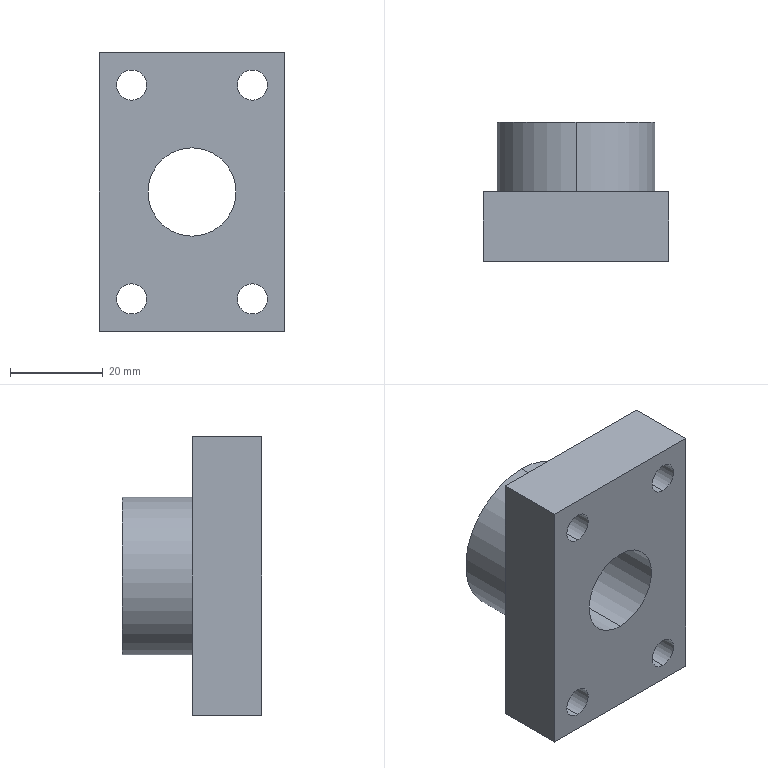Part | STEP file | 1 solid | 19 faces | box 40 x 30 x 60 mm | volume 39122 mm3 | cylinder 12 | plane 7 | commonest cylinder face diameters 6.5 x8 19 x2 34 x2
STEP:
#1=CARTESIAN_POINT('',(0.,0.,0.));
#2=DIRECTION('',(0.,0.,1.));
#3=DIRECTION('',(1.,0.,0.));
#4=AXIS2_PLACEMENT_3D('',#1,#2,#3);
#5=CARTESIAN_POINT('',(-13.,0.,-19.75));
#6=VERTEX_POINT('',#5);
#7=CARTESIAN_POINT('',(-13.,15.,-19.75));
#8=VERTEX_POINT('',#7);
#9=CARTESIAN_POINT('',(-13.,15.,-19.75));
#10=DIRECTION('',(0.,1.,0.));
#11=VECTOR('',#10,1.);
#12=LINE('',#9,#11);
#13=CARTESIAN_POINT('',(-13.,15.,-23.));
#14=DIRECTION('',(0.,1.,0.));
#15=DIRECTION('',(0.,0.,1.));
#16=AXIS2_PLACEMENT_3D('',#13,#14,#15);
#17=CYLINDRICAL_SURFACE('',#16,3.25);
#18=CARTESIAN_POINT('',(6.283,0.));
#19=DIRECTION('',(0.,1.));
#20=VECTOR('',#19,1.);
#21=LINE('',#18,#20);
#22=(GEOMETRIC_REPRESENTATION_CONTEXT(2)PARAMETRIC_REPRESENTATION_CONTEXT()REPRESENTATION_CONTEXT('',''));
#23=DEFINITIONAL_REPRESENTATION('',(#21),#22);
#24=PCURVE('',#17,#23);
#25=CARTESIAN_POINT('',(-13.,15.,-23.));
#26=DIRECTION('',(0.,1.,0.));
#27=DIRECTION('',(0.,0.,1.));
#28=AXIS2_PLACEMENT_3D('',#25,#26,#27);
#29=CYLINDRICAL_SURFACE('',#28,3.25);
#30=CARTESIAN_POINT('',(0.,0.));
#31=DIRECTION('',(0.,1.));
#32=VECTOR('',#31,1.);
#33=LINE('',#30,#32);
#34=(GEOMETRIC_REPRESENTATION_CONTEXT(2)PARAMETRIC_REPRESENTATION_CONTEXT()REPRESENTATION_CONTEXT('',''));
#35=DEFINITIONAL_REPRESENTATION('',(#33),#34);
#36=PCURVE('',#29,#35);
#37=SURFACE_CURVE('',#12,(#24,#36),.PCURVE_S1.);
#38=EDGE_CURVE('',#6,#8,#37,.T.);
#39=ORIENTED_EDGE('',*,*,#38,.T.);
#40=CARTESIAN_POINT('',(-13.,15.,-26.25));
#41=VERTEX_POINT('',#40);
#42=CARTESIAN_POINT('',(-13.,15.,-23.));
#43=DIRECTION('',(0.,1.,0.));
#44=DIRECTION('',(0.,0.,1.));
#45=AXIS2_PLACEMENT_3D('',#42,#43,#44);
#46=CIRCLE('',#45,3.25);
#47=CARTESIAN_POINT('',(0.,0.));
#48=DIRECTION('',(1.,0.));
#49=VECTOR('',#48,1.);
#50=LINE('',#47,#49);
#51=(GEOMETRIC_REPRESENTATION_CONTEXT(2)PARAMETRIC_REPRESENTATION_CONTEXT()REPRESENTATION_CONTEXT('',''));
#52=DEFINITIONAL_REPRESENTATION('',(#50),#51);
#53=PCURVE('',#17,#52);
#54=CARTESIAN_POINT('',(0.,15.,0.));
#55=DIRECTION('',(0.,1.,0.));
#56=DIRECTION('',(0.,0.,1.));
#57=AXIS2_PLACEMENT_3D('',#54,#55,#56);
#58=PLANE('',#57);
#59=CARTESIAN_POINT('',(-23.,-13.));
#60=DIRECTION('',(1.,0.));
#61=AXIS2_PLACEMENT_2D('',#59,#60);
#62=CIRCLE('',#61,3.25);
#63=(GEOMETRIC_REPRESENTATION_CONTEXT(2)PARAMETRIC_REPRESENTATION_CONTEXT()REPRESENTATION_CONTEXT('',''));
#64=DEFINITIONAL_REPRESENTATION('',(#62),#63);
#65=PCURVE('',#58,#64);
#66=SURFACE_CURVE('',#46,(#53,#65),.PCURVE_S1.);
#67=EDGE_CURVE('',#41,#8,#66,.T.);
#68=ORIENTED_EDGE('',*,*,#67,.F.);
#69=CARTESIAN_POINT('',(-13.,0.,-26.25));
#70=VERTEX_POINT('',#69);
#71=CARTESIAN_POINT('',(-13.,15.,-26.25));
#72=DIRECTION('',(0.,1.,0.));
#73=VECTOR('',#72,1.);
#74=LINE('',#71,#73);
#75=CARTESIAN_POINT('',(3.142,0.));
#76=DIRECTION('',(0.,1.));
#77=VECTOR('',#76,1.);
#78=LINE('',#75,#77);
#79=(GEOMETRIC_REPRESENTATION_CONTEXT(2)PARAMETRIC_REPRESENTATION_CONTEXT()REPRESENTATION_CONTEXT('',''));
#80=DEFINITIONAL_REPRESENTATION('',(#78),#79);
#81=PCURVE('',#17,#80);
#82=CARTESIAN_POINT('',(3.142,0.));
#83=DIRECTION('',(0.,1.));
#84=VECTOR('',#83,1.);
#85=LINE('',#82,#84);
#86=(GEOMETRIC_REPRESENTATION_CONTEXT(2)PARAMETRIC_REPRESENTATION_CONTEXT()REPRESENTATION_CONTEXT('',''));
#87=DEFINITIONAL_REPRESENTATION('',(#85),#86);
#88=PCURVE('',#29,#87);
#89=SURFACE_CURVE('',#74,(#81,#88),.PCURVE_S1.);
#90=EDGE_CURVE('',#70,#41,#89,.T.);
#91=ORIENTED_EDGE('',*,*,#90,.F.);
#92=CARTESIAN_POINT('',(-13.,0.,-23.));
#93=DIRECTION('',(0.,1.,0.));
#94=DIRECTION('',(0.,0.,1.));
#95=AXIS2_PLACEMENT_3D('',#92,#93,#94);
#96=CIRCLE('',#95,3.25);
#97=CARTESIAN_POINT('',(0.,-15.));
#98=DIRECTION('',(1.,0.));
#99=VECTOR('',#98,1.);
#100=LINE('',#97,#99);
#101=(GEOMETRIC_REPRESENTATION_CONTEXT(2)PARAMETRIC_REPRESENTATION_CONTEXT()REPRESENTATION_CONTEXT('',''));
#102=DEFINITIONAL_REPRESENTATION('',(#100),#101);
#103=PCURVE('',#17,#102);
#104=CARTESIAN_POINT('',(0.,0.,0.));
#105=DIRECTION('',(0.,1.,0.));
#106=DIRECTION('',(0.,0.,1.));
#107=AXIS2_PLACEMENT_3D('',#104,#105,#106);
#108=PLANE('',#107);
#109=CARTESIAN_POINT('',(-23.,-13.));
#110=DIRECTION('',(1.,0.));
#111=AXIS2_PLACEMENT_2D('',#109,#110);
#112=CIRCLE('',#111,3.25);
#113=(GEOMETRIC_REPRESENTATION_CONTEXT(2)PARAMETRIC_REPRESENTATION_CONTEXT()REPRESENTATION_CONTEXT('',''));
#114=DEFINITIONAL_REPRESENTATION('',(#112),#113);
#115=PCURVE('',#108,#114);
#116=SURFACE_CURVE('',#96,(#103,#115),.PCURVE_S1.);
#117=EDGE_CURVE('',#70,#6,#116,.T.);
#118=ORIENTED_EDGE('',*,*,#117,.T.);
#119=EDGE_LOOP('',(#39,#68,#91,#118));
#120=FACE_BOUND('',#119,.F.);
#121=ADVANCED_FACE('',(#120),#17,.F.);
#122=CARTESIAN_POINT('',(13.,0.,-19.75));
#123=VERTEX_POINT('',#122);
#124=CARTESIAN_POINT('',(13.,15.,-19.75));
#125=VERTEX_POINT('',#124);
#126=CARTESIAN_POINT('',(13.,15.,-19.75));
#127=DIRECTION('',(0.,1.,0.));
#128=VECTOR('',#127,1.);
#129=LINE('',#126,#128);
#130=CARTESIAN_POINT('',(13.,15.,-23.));
#131=DIRECTION('',(0.,1.,0.));
#132=DIRECTION('',(0.,0.,1.));
#133=AXIS2_PLACEMENT_3D('',#130,#131,#132);
#134=CYLINDRICAL_SURFACE('',#133,3.25);
#135=CARTESIAN_POINT('',(6.283,0.));
#136=DIRECTION('',(0.,1.));
#137=VECTOR('',#136,1.);
#138=LINE('',#135,#137);
#139=(GEOMETRIC_REPRESENTATION_CONTEXT(2)PARAMETRIC_REPRESENTATION_CONTEXT()REPRESENTATION_CONTEXT('',''));
#140=DEFINITIONAL_REPRESENTATION('',(#138),#139);
#141=PCURVE('',#134,#140);
#142=CARTESIAN_POINT('',(13.,15.,-23.));
#143=DIRECTION('',(0.,1.,0.));
#144=DIRECTION('',(0.,0.,1.));
#145=AXIS2_PLACEMENT_3D('',#142,#143,#144);
#146=CYLINDRICAL_SURFACE('',#145,3.25);
#147=CARTESIAN_POINT('',(0.,0.));
#148=DIRECTION('',(0.,1.));
#149=VECTOR('',#148,1.);
#150=LINE('',#147,#149);
#151=(GEOMETRIC_REPRESENTATION_CONTEXT(2)PARAMETRIC_REPRESENTATION_CONTEXT()REPRESENTATION_CONTEXT('',''));
#152=DEFINITIONAL_REPRESENTATION('',(#150),#151);
#153=PCURVE('',#146,#152);
#154=SURFACE_CURVE('',#129,(#141,#153),.PCURVE_S1.);
#155=EDGE_CURVE('',#123,#125,#154,.T.);
#156=ORIENTED_EDGE('',*,*,#155,.T.);
#157=CARTESIAN_POINT('',(13.,15.,-26.25));
#158=VERTEX_POINT('',#157);
#159=CARTESIAN_POINT('',(13.,15.,-23.));
#160=DIRECTION('',(0.,1.,0.));
#161=DIRECTION('',(0.,0.,1.));
#162=AXIS2_PLACEMENT_3D('',#159,#160,#161);
#163=CIRCLE('',#162,3.25);
#164=CARTESIAN_POINT('',(0.,0.));
#165=DIRECTION('',(1.,0.));
#166=VECTOR('',#165,1.);
#167=LINE('',#164,#166);
#168=(GEOMETRIC_REPRESENTATION_CONTEXT(2)PARAMETRIC_REPRESENTATION_CONTEXT()REPRESENTATION_CONTEXT('',''));
#169=DEFINITIONAL_REPRESENTATION('',(#167),#168);
#170=PCURVE('',#134,#169);
#171=CARTESIAN_POINT('',(-23.,13.));
#172=DIRECTION('',(1.,0.));
#173=AXIS2_PLACEMENT_2D('',#171,#172);
#174=CIRCLE('',#173,3.25);
#175=(GEOMETRIC_REPRESENTATION_CONTEXT(2)PARAMETRIC_REPRESENTATION_CONTEXT()REPRESENTATION_CONTEXT('',''));
#176=DEFINITIONAL_REPRESENTATION('',(#174),#175);
#177=PCURVE('',#58,#176);
#178=SURFACE_CURVE('',#163,(#170,#177),.PCURVE_S1.);
#179=EDGE_CURVE('',#158,#125,#178,.T.);
#180=ORIENTED_EDGE('',*,*,#179,.F.);
#181=CARTESIAN_POINT('',(13.,0.,-26.25));
#182=VERTEX_POINT('',#181);
#183=CARTESIAN_POINT('',(13.,15.,-26.25));
#184=DIRECTION('',(0.,1.,0.));
#185=VECTOR('',#184,1.);
#186=LINE('',#183,#185);
#187=CARTESIAN_POINT('',(3.142,0.));
#188=DIRECTION('',(0.,1.));
#189=VECTOR('',#188,1.);
#190=LINE('',#187,#189);
#191=(GEOMETRIC_REPRESENTATION_CONTEXT(2)PARAMETRIC_REPRESENTATION_CONTEXT()REPRESENTATION_CONTEXT('',''));
#192=DEFINITIONAL_REPRESENTATION('',(#190),#191);
#193=PCURVE('',#134,#192);
#194=CARTESIAN_POINT('',(3.142,0.));
#195=DIRECTION('',(0.,1.));
#196=VECTOR('',#195,1.);
#197=LINE('',#194,#196);
#198=(GEOMETRIC_REPRESENTATION_CONTEXT(2)PARAMETRIC_REPRESENTATION_CONTEXT()REPRESENTATION_CONTEXT('',''));
#199=DEFINITIONAL_REPRESENTATION('',(#197),#198);
#200=PCURVE('',#146,#199);
#201=SURFACE_CURVE('',#186,(#193,#200),.PCURVE_S1.);
#202=EDGE_CURVE('',#182,#158,#201,.T.);
#203=ORIENTED_EDGE('',*,*,#202,.F.);
#204=CARTESIAN_POINT('',(13.,0.,-23.));
#205=DIRECTION('',(0.,1.,0.));
#206=DIRECTION('',(0.,0.,1.));
#207=AXIS2_PLACEMENT_3D('',#204,#205,#206);
#208=CIRCLE('',#207,3.25);
#209=CARTESIAN_POINT('',(0.,-15.));
#210=DIRECTION('',(1.,0.));
#211=VECTOR('',#210,1.);
#212=LINE('',#209,#211);
#213=(GEOMETRIC_REPRESENTATION_CONTEXT(2)PARAMETRIC_REPRESENTATION_CONTEXT()REPRESENTATION_CONTEXT('',''));
#214=DEFINITIONAL_REPRESENTATION('',(#212),#213);
#215=PCURVE('',#134,#214);
#216=CARTESIAN_POINT('',(-23.,13.));
#217=DIRECTION('',(1.,0.));
#218=AXIS2_PLACEMENT_2D('',#216,#217);
#219=CIRCLE('',#218,3.25);
#220=(GEOMETRIC_REPRESENTATION_CONTEXT(2)PARAMETRIC_REPRESENTATION_CONTEXT()REPRESENTATION_CONTEXT('',''));
#221=DEFINITIONAL_REPRESENTATION('',(#219),#220);
#222=PCURVE('',#108,#221);
#223=SURFACE_CURVE('',#208,(#215,#222),.PCURVE_S1.);
#224=EDGE_CURVE('',#182,#123,#223,.T.);
#225=ORIENTED_EDGE('',*,*,#224,.T.);
#226=EDGE_LOOP('',(#156,#180,#203,#225));
#227=FACE_BOUND('',#226,.F.);
#228=ADVANCED_FACE('',(#227),#134,.F.);
#229=CARTESIAN_POINT('',(13.,0.,26.25));
#230=VERTEX_POINT('',#229);
#231=CARTESIAN_POINT('',(13.,15.,26.25));
#232=VERTEX_POINT('',#231);
#233=CARTESIAN_POINT('',(13.,15.,26.25));
#234=DIRECTION('',(0.,1.,0.));
#235=VECTOR('',#234,1.);
#236=LINE('',#233,#235);
#237=CARTESIAN_POINT('',(13.,15.,23.));
#238=DIRECTION('',(0.,1.,0.));
#239=DIRECTION('',(0.,0.,1.));
#240=AXIS2_PLACEMENT_3D('',#237,#238,#239);
#241=CYLINDRICAL_SURFACE('',#240,3.25);
#242=CARTESIAN_POINT('',(6.283,0.));
#243=DIRECTION('',(0.,1.));
#244=VECTOR('',#243,1.);
#245=LINE('',#242,#244);
#246=(GEOMETRIC_REPRESENTATION_CONTEXT(2)PARAMETRIC_REPRESENTATION_CONTEXT()REPRESENTATION_CONTEXT('',''));
#247=DEFINITIONAL_REPRESENTATION('',(#245),#246);
#248=PCURVE('',#241,#247);
#249=CARTESIAN_POINT('',(13.,15.,23.));
#250=DIRECTION('',(0.,1.,0.));
#251=DIRECTION('',(0.,0.,1.));
#252=AXIS2_PLACEMENT_3D('',#249,#250,#251);
#253=CYLINDRICAL_SURFACE('',#252,3.25);
#254=CARTESIAN_POINT('',(0.,0.));
#255=DIRECTION('',(0.,1.));
#256=VECTOR('',#255,1.);
#257=LINE('',#254,#256);
#258=(GEOMETRIC_REPRESENTATION_CONTEXT(2)PARAMETRIC_REPRESENTATION_CONTEXT()REPRESENTATION_CONTEXT('',''));
#259=DEFINITIONAL_REPRESENTATION('',(#257),#258);
#260=PCURVE('',#253,#259);
#261=SURFACE_CURVE('',#236,(#248,#260),.PCURVE_S1.);
#262=EDGE_CURVE('',#230,#232,#261,.T.);
#263=ORIENTED_EDGE('',*,*,#262,.T.);
#264=CARTESIAN_POINT('',(13.,15.,19.75));
#265=VERTEX_POINT('',#264);
#266=CARTESIAN_POINT('',(13.,15.,23.));
#267=DIRECTION('',(0.,1.,0.));
#268=DIRECTION('',(0.,0.,1.));
#269=AXIS2_PLACEMENT_3D('',#266,#267,#268);
#270=CIRCLE('',#269,3.25);
#271=CARTESIAN_POINT('',(0.,0.));
#272=DIRECTION('',(1.,0.));
#273=VECTOR('',#272,1.);
#274=LINE('',#271,#273);
#275=(GEOMETRIC_REPRESENTATION_CONTEXT(2)PARAMETRIC_REPRESENTATION_CONTEXT()REPRESENTATION_CONTEXT('',''));
#276=DEFINITIONAL_REPRESENTATION('',(#274),#275);
#277=PCURVE('',#241,#276);
#278=CARTESIAN_POINT('',(23.,13.));
#279=DIRECTION('',(1.,0.));
#280=AXIS2_PLACEMENT_2D('',#278,#279);
#281=CIRCLE('',#280,3.25);
#282=(GEOMETRIC_REPRESENTATION_CONTEXT(2)PARAMETRIC_REPRESENTATION_CONTEXT()REPRESENTATION_CONTEXT('',''));
#283=DEFINITIONAL_REPRESENTATION('',(#281),#282);
#284=PCURVE('',#58,#283);
#285=SURFACE_CURVE('',#270,(#277,#284),.PCURVE_S1.);
#286=EDGE_CURVE('',#265,#232,#285,.T.);
#287=ORIENTED_EDGE('',*,*,#286,.F.);
#288=CARTESIAN_POINT('',(13.,0.,19.75));
#289=VERTEX_POINT('',#288);
#290=CARTESIAN_POINT('',(13.,15.,19.75));
#291=DIRECTION('',(0.,1.,0.));
#292=VECTOR('',#291,1.);
#293=LINE('',#290,#292);
#294=CARTESIAN_POINT('',(3.142,0.));
#295=DIRECTION('',(0.,1.));
#296=VECTOR('',#295,1.);
#297=LINE('',#294,#296);
#298=(GEOMETRIC_REPRESENTATION_CONTEXT(2)PARAMETRIC_REPRESENTATION_CONTEXT()REPRESENTATION_CONTEXT('',''));
#299=DEFINITIONAL_REPRESENTATION('',(#297),#298);
#300=PCURVE('',#241,#299);
#301=CARTESIAN_POINT('',(3.142,0.));
#302=DIRECTION('',(0.,1.));
#303=VECTOR('',#302,1.);
#304=LINE('',#301,#303);
#305=(GEOMETRIC_REPRESENTATION_CONTEXT(2)PARAMETRIC_REPRESENTATION_CONTEXT()REPRESENTATION_CONTEXT('',''));
#306=DEFINITIONAL_REPRESENTATION('',(#304),#305);
#307=PCURVE('',#253,#306);
#308=SURFACE_CURVE('',#293,(#300,#307),.PCURVE_S1.);
#309=EDGE_CURVE('',#289,#265,#308,.T.);
#310=ORIENTED_EDGE('',*,*,#309,.F.);
#311=CARTESIAN_POINT('',(13.,0.,23.));
#312=DIRECTION('',(0.,1.,0.));
#313=DIRECTION('',(0.,0.,1.));
#314=AXIS2_PLACEMENT_3D('',#311,#312,#313);
#315=CIRCLE('',#314,3.25);
#316=CARTESIAN_POINT('',(0.,-15.));
#317=DIRECTION('',(1.,0.));
#318=VECTOR('',#317,1.);
#319=LINE('',#316,#318);
#320=(GEOMETRIC_REPRESENTATION_CONTEXT(2)PARAMETRIC_REPRESENTATION_CONTEXT()REPRESENTATION_CONTEXT('',''));
#321=DEFINITIONAL_REPRESENTATION('',(#319),#320);
#322=PCURVE('',#241,#321);
#323=CARTESIAN_POINT('',(23.,13.));
#324=DIRECTION('',(1.,0.));
#325=AXIS2_PLACEMENT_2D('',#323,#324);
#326=CIRCLE('',#325,3.25);
#327=(GEOMETRIC_REPRESENTATION_CONTEXT(2)PARAMETRIC_REPRESENTATION_CONTEXT()REPRESENTATION_CONTEXT('',''));
#328=DEFINITIONAL_REPRESENTATION('',(#326),#327);
#329=PCURVE('',#108,#328);
#330=SURFACE_CURVE('',#315,(#322,#329),.PCURVE_S1.);
#331=EDGE_CURVE('',#289,#230,#330,.T.);
#332=ORIENTED_EDGE('',*,*,#331,.T.);
#333=EDGE_LOOP('',(#263,#287,#310,#332));
#334=FACE_BOUND('',#333,.F.);
#335=ADVANCED_FACE('',(#334),#241,.F.);
#336=CARTESIAN_POINT('',(-13.,0.,26.25));
#337=VERTEX_POINT('',#336);
#338=CARTESIAN_POINT('',(-13.,15.,26.25));
#339=VERTEX_POINT('',#338);
#340=CARTESIAN_POINT('',(-13.,15.,26.25));
#341=DIRECTION('',(0.,1.,0.));
#342=VECTOR('',#341,1.);
#343=LINE('',#340,#342);
#344=CARTESIAN_POINT('',(-13.,15.,23.));
#345=DIRECTION('',(0.,1.,0.));
#346=DIRECTION('',(0.,0.,1.));
#347=AXIS2_PLACEMENT_3D('',#344,#345,#346);
#348=CYLINDRICAL_SURFACE('',#347,3.25);
#349=CARTESIAN_POINT('',(6.283,0.));
#350=DIRECTION('',(0.,1.));
#351=VECTOR('',#350,1.);
#352=LINE('',#349,#351);
#353=(GEOMETRIC_REPRESENTATION_CONTEXT(2)PARAMETRIC_REPRESENTATION_CONTEXT()REPRESENTATION_CONTEXT('',''));
#354=DEFINITIONAL_REPRESENTATION('',(#352),#353);
#355=PCURVE('',#348,#354);
#356=CARTESIAN_POINT('',(-13.,15.,23.));
#357=DIRECTION('',(0.,1.,0.));
#358=DIRECTION('',(0.,0.,1.));
#359=AXIS2_PLACEMENT_3D('',#356,#357,#358);
#360=CYLINDRICAL_SURFACE('',#359,3.25);
#361=CARTESIAN_POINT('',(0.,0.));
#362=DIRECTION('',(0.,1.));
#363=VECTOR('',#362,1.);
#364=LINE('',#361,#363);
#365=(GEOMETRIC_REPRESENTATION_CONTEXT(2)PARAMETRIC_REPRESENTATION_CONTEXT()REPRESENTATION_CONTEXT('',''));
#366=DEFINITIONAL_REPRESENTATION('',(#364),#365);
#367=PCURVE('',#360,#366);
#368=SURFACE_CURVE('',#343,(#355,#367),.PCURVE_S1.);
#369=EDGE_CURVE('',#337,#339,#368,.T.);
#370=ORIENTED_EDGE('',*,*,#369,.T.);
#371=CARTESIAN_POINT('',(-13.,15.,19.75));
#372=VERTEX_POINT('',#371);
#373=CARTESIAN_POINT('',(-13.,15.,23.));
#374=DIRECTION('',(0.,1.,0.));
#375=DIRECTION('',(0.,0.,1.));
#376=AXIS2_PLACEMENT_3D('',#373,#374,#375);
#377=CIRCLE('',#376,3.25);
#378=CARTESIAN_POINT('',(0.,0.));
#379=DIRECTION('',(1.,0.));
#380=VECTOR('',#379,1.);
#381=LINE('',#378,#380);
#382=(GEOMETRIC_REPRESENTATION_CONTEXT(2)PARAMETRIC_REPRESENTATION_CONTEXT()REPRESENTATION_CONTEXT('',''));
#383=DEFINITIONAL_REPRESENTATION('',(#381),#382);
#384=PCURVE('',#348,#383);
#385=CARTESIAN_POINT('',(23.,-13.));
#386=DIRECTION('',(1.,0.));
#387=AXIS2_PLACEMENT_2D('',#385,#386);
#388=CIRCLE('',#387,3.25);
#389=(GEOMETRIC_REPRESENTATION_CONTEXT(2)PARAMETRIC_REPRESENTATION_CONTEXT()REPRESENTATION_CONTEXT('',''));
#390=DEFINITIONAL_REPRESENTATION('',(#388),#389);
#391=PCURVE('',#58,#390);
#392=SURFACE_CURVE('',#377,(#384,#391),.PCURVE_S1.);
#393=EDGE_CURVE('',#372,#339,#392,.T.);
#394=ORIENTED_EDGE('',*,*,#393,.F.);
#395=CARTESIAN_POINT('',(-13.,0.,19.75));
#396=VERTEX_POINT('',#395);
#397=CARTESIAN_POINT('',(-13.,15.,19.75));
#398=DIRECTION('',(0.,1.,0.));
#399=VECTOR('',#398,1.);
#400=LINE('',#397,#399);
#401=CARTESIAN_POINT('',(3.142,0.));
#402=DIRECTION('',(0.,1.));
#403=VECTOR('',#402,1.);
#404=LINE('',#401,#403);
#405=(GEOMETRIC_REPRESENTATION_CONTEXT(2)PARAMETRIC_REPRESENTATION_CONTEXT()REPRESENTATION_CONTEXT('',''));
#406=DEFINITIONAL_REPRESENTATION('',(#404),#405);
#407=PCURVE('',#348,#406);
#408=CARTESIAN_POINT('',(3.142,0.));
#409=DIRECTION('',(0.,1.));
#410=VECTOR('',#409,1.);
#411=LINE('',#408,#410);
#412=(GEOMETRIC_REPRESENTATION_CONTEXT(2)PARAMETRIC_REPRESENTATION_CONTEXT()REPRESENTATION_CONTEXT('',''));
#413=DEFINITIONAL_REPRESENTATION('',(#411),#412);
#414=PCURVE('',#360,#413);
#415=SURFACE_CURVE('',#400,(#407,#414),.PCURVE_S1.);
#416=EDGE_CURVE('',#396,#372,#415,.T.);
#417=ORIENTED_EDGE('',*,*,#416,.F.);
#418=CARTESIAN_POINT('',(-13.,0.,23.));
#419=DIRECTION('',(0.,1.,0.));
#420=DIRECTION('',(0.,0.,1.));
#421=AXIS2_PLACEMENT_3D('',#418,#419,#420);
#422=CIRCLE('',#421,3.25);
#423=CARTESIAN_POINT('',(0.,-15.));
#424=DIRECTION('',(1.,0.));
#425=VECTOR('',#424,1.);
#426=LINE('',#423,#425);
#427=(GEOMETRIC_REPRESENTATION_CONTEXT(2)PARAMETRIC_REPRESENTATION_CONTEXT()REPRESENTATION_CONTEXT('',''));
#428=DEFINITIONAL_REPRESENTATION('',(#426),#427);
#429=PCURVE('',#348,#428);
#430=CARTESIAN_POINT('',(23.,-13.));
#431=DIRECTION('',(1.,0.));
#432=AXIS2_PLACEMENT_2D('',#430,#431);
#433=CIRCLE('',#432,3.25);
#434=(GEOMETRIC_REPRESENTATION_CONTEXT(2)PARAMETRIC_REPRESENTATION_CONTEXT()REPRESENTATION_CONTEXT('',''));
#435=DEFINITIONAL_REPRESENTATION('',(#433),#434);
#436=PCURVE('',#108,#435);
#437=SURFACE_CURVE('',#422,(#429,#436),.PCURVE_S1.);
#438=EDGE_CURVE('',#396,#337,#437,.T.);
#439=ORIENTED_EDGE('',*,*,#438,.T.);
#440=EDGE_LOOP('',(#370,#394,#417,#439));
#441=FACE_BOUND('',#440,.F.);
#442=ADVANCED_FACE('',(#441),#348,.F.);
#443=CARTESIAN_POINT('',(0.,0.,9.5));
#444=VERTEX_POINT('',#443);
#445=CARTESIAN_POINT('',(0.,30.,9.5));
#446=VERTEX_POINT('',#445);
#447=CARTESIAN_POINT('',(0.,0.,9.5));
#448=DIRECTION('',(0.,1.,0.));
#449=VECTOR('',#448,1.);
#450=LINE('',#447,#449);
#451=CARTESIAN_POINT('',(0.,0.,0.));
#452=DIRECTION('',(0.,1.,0.));
#453=DIRECTION('',(0.,0.,1.));
#454=AXIS2_PLACEMENT_3D('',#451,#452,#453);
#455=CYLINDRICAL_SURFACE('',#454,9.5);
#456=CARTESIAN_POINT('',(6.283,0.));
#457=DIRECTION('',(0.,1.));
#458=VECTOR('',#457,1.);
#459=LINE('',#456,#458);
#460=(GEOMETRIC_REPRESENTATION_CONTEXT(2)PARAMETRIC_REPRESENTATION_CONTEXT()REPRESENTATION_CONTEXT('',''));
#461=DEFINITIONAL_REPRESENTATION('',(#459),#460);
#462=PCURVE('',#455,#461);
#463=CARTESIAN_POINT('',(0.,0.,0.));
#464=DIRECTION('',(0.,1.,0.));
#465=DIRECTION('',(0.,0.,1.));
#466=AXIS2_PLACEMENT_3D('',#463,#464,#465);
#467=CYLINDRICAL_SURFACE('',#466,9.5);
#468=CARTESIAN_POINT('',(0.,0.));
#469=DIRECTION('',(0.,1.));
#470=VECTOR('',#469,1.);
#471=LINE('',#468,#470);
#472=(GEOMETRIC_REPRESENTATION_CONTEXT(2)PARAMETRIC_REPRESENTATION_CONTEXT()REPRESENTATION_CONTEXT('',''));
#473=DEFINITIONAL_REPRESENTATION('',(#471),#472);
#474=PCURVE('',#467,#473);
#475=SURFACE_CURVE('',#450,(#462,#474),.PCURVE_S1.);
#476=EDGE_CURVE('',#444,#446,#475,.T.);
#477=ORIENTED_EDGE('',*,*,#476,.T.);
#478=CARTESIAN_POINT('',(0.,30.,-9.5));
#479=VERTEX_POINT('',#478);
#480=CARTESIAN_POINT('',(0.,30.,0.));
#481=DIRECTION('',(0.,1.,0.));
#482=DIRECTION('',(0.,0.,1.));
#483=AXIS2_PLACEMENT_3D('',#480,#481,#482);
#484=CIRCLE('',#483,9.5);
#485=CARTESIAN_POINT('',(0.,30.));
#486=DIRECTION('',(1.,0.));
#487=VECTOR('',#486,1.);
#488=LINE('',#485,#487);
#489=(GEOMETRIC_REPRESENTATION_CONTEXT(2)PARAMETRIC_REPRESENTATION_CONTEXT()REPRESENTATION_CONTEXT('',''));
#490=DEFINITIONAL_REPRESENTATION('',(#488),#489);
#491=PCURVE('',#455,#490);
#492=CARTESIAN_POINT('',(0.,30.,0.));
#493=DIRECTION('',(0.,1.,0.));
#494=DIRECTION('',(0.,0.,1.));
#495=AXIS2_PLACEMENT_3D('',#492,#493,#494);
#496=PLANE('',#495);
#497=CARTESIAN_POINT('',(0.,0.));
#498=DIRECTION('',(1.,0.));
#499=AXIS2_PLACEMENT_2D('',#497,#498);
#500=CIRCLE('',#499,9.5);
#501=(GEOMETRIC_REPRESENTATION_CONTEXT(2)PARAMETRIC_REPRESENTATION_CONTEXT()REPRESENTATION_CONTEXT('',''));
#502=DEFINITIONAL_REPRESENTATION('',(#500),#501);
#503=PCURVE('',#496,#502);
#504=SURFACE_CURVE('',#484,(#491,#503),.PCURVE_S1.);
#505=EDGE_CURVE('',#479,#446,#504,.T.);
#506=ORIENTED_EDGE('',*,*,#505,.F.);
#507=CARTESIAN_POINT('',(0.,0.,-9.5));
#508=VERTEX_POINT('',#507);
#509=CARTESIAN_POINT('',(0.,0.,-9.5));
#510=DIRECTION('',(0.,1.,0.));
#511=VECTOR('',#510,1.);
#512=LINE('',#509,#511);
#513=CARTESIAN_POINT('',(3.142,0.));
#514=DIRECTION('',(0.,1.));
#515=VECTOR('',#514,1.);
#516=LINE('',#513,#515);
#517=(GEOMETRIC_REPRESENTATION_CONTEXT(2)PARAMETRIC_REPRESENTATION_CONTEXT()REPRESENTATION_CONTEXT('',''));
#518=DEFINITIONAL_REPRESENTATION('',(#516),#517);
#519=PCURVE('',#455,#518);
#520=CARTESIAN_POINT('',(3.142,0.));
#521=DIRECTION('',(0.,1.));
#522=VECTOR('',#521,1.);
#523=LINE('',#520,#522);
#524=(GEOMETRIC_REPRESENTATION_CONTEXT(2)PARAMETRIC_REPRESENTATION_CONTEXT()REPRESENTATION_CONTEXT('',''));
#525=DEFINITIONAL_REPRESENTATION('',(#523),#524);
#526=PCURVE('',#467,#525);
#527=SURFACE_CURVE('',#512,(#519,#526),.PCURVE_S1.);
#528=EDGE_CURVE('',#508,#479,#527,.T.);
#529=ORIENTED_EDGE('',*,*,#528,.F.);
#530=CARTESIAN_POINT('',(0.,0.,0.));
#531=DIRECTION('',(0.,1.,0.));
#532=DIRECTION('',(0.,0.,1.));
#533=AXIS2_PLACEMENT_3D('',#530,#531,#532);
#534=CIRCLE('',#533,9.5);
#535=CARTESIAN_POINT('',(0.,0.));
#536=DIRECTION('',(1.,0.));
#537=VECTOR('',#536,1.);
#538=LINE('',#535,#537);
#539=(GEOMETRIC_REPRESENTATION_CONTEXT(2)PARAMETRIC_REPRESENTATION_CONTEXT()REPRESENTATION_CONTEXT('',''));
#540=DEFINITIONAL_REPRESENTATION('',(#538),#539);
#541=PCURVE('',#455,#540);
#542=CARTESIAN_POINT('',(0.,0.));
#543=DIRECTION('',(1.,0.));
#544=AXIS2_PLACEMENT_2D('',#542,#543);
#545=CIRCLE('',#544,9.5);
#546=(GEOMETRIC_REPRESENTATION_CONTEXT(2)PARAMETRIC_REPRESENTATION_CONTEXT()REPRESENTATION_CONTEXT('',''));
#547=DEFINITIONAL_REPRESENTATION('',(#545),#546);
#548=PCURVE('',#108,#547);
#549=SURFACE_CURVE('',#534,(#541,#548),.PCURVE_S1.);
#550=EDGE_CURVE('',#508,#444,#549,.T.);
#551=ORIENTED_EDGE('',*,*,#550,.T.);
#552=EDGE_LOOP('',(#477,#506,#529,#551));
#553=FACE_BOUND('',#552,.F.);
#554=ADVANCED_FACE('',(#553),#455,.F.);
#555=CARTESIAN_POINT('',(0.,30.,17.));
#556=VERTEX_POINT('',#555);
#557=CARTESIAN_POINT('',(0.,30.,-17.));
#558=VERTEX_POINT('',#557);
#559=CARTESIAN_POINT('',(0.,30.,0.));
#560=DIRECTION('',(0.,1.,0.));
#561=DIRECTION('',(0.,0.,1.));
#562=AXIS2_PLACEMENT_3D('',#559,#560,#561);
#563=CIRCLE('',#562,17.);
#564=CARTESIAN_POINT('',(0.,30.,0.));
#565=DIRECTION('',(0.,-1.,0.));
#566=DIRECTION('',(0.,0.,-1.));
#567=AXIS2_PLACEMENT_3D('',#564,#565,#566);
#568=CYLINDRICAL_SURFACE('',#567,17.);
#569=CARTESIAN_POINT('',(3.142,0.));
#570=DIRECTION('',(-1.,0.));
#571=VECTOR('',#570,1.);
#572=LINE('',#569,#571);
#573=(GEOMETRIC_REPRESENTATION_CONTEXT(2)PARAMETRIC_REPRESENTATION_CONTEXT()REPRESENTATION_CONTEXT('',''));
#574=DEFINITIONAL_REPRESENTATION('',(#572),#573);
#575=PCURVE('',#568,#574);
#576=CARTESIAN_POINT('',(0.,0.));
#577=DIRECTION('',(1.,0.));
#578=AXIS2_PLACEMENT_2D('',#576,#577);
#579=CIRCLE('',#578,17.);
#580=(GEOMETRIC_REPRESENTATION_CONTEXT(2)PARAMETRIC_REPRESENTATION_CONTEXT()REPRESENTATION_CONTEXT('',''));
#581=DEFINITIONAL_REPRESENTATION('',(#579),#580);
#582=PCURVE('',#496,#581);
#583=SURFACE_CURVE('',#563,(#575,#582),.PCURVE_S1.);
#584=EDGE_CURVE('',#556,#558,#583,.T.);
#585=ORIENTED_EDGE('',*,*,#584,.F.);
#586=CARTESIAN_POINT('',(0.,15.,17.));
#587=VERTEX_POINT('',#586);
#588=CARTESIAN_POINT('',(0.,30.,17.));
#589=DIRECTION('',(0.,-1.,0.));
#590=VECTOR('',#589,1.);
#591=LINE('',#588,#590);
#592=CARTESIAN_POINT('',(3.142,0.));
#593=DIRECTION('',(0.,1.));
#594=VECTOR('',#593,1.);
#595=LINE('',#592,#594);
#596=(GEOMETRIC_REPRESENTATION_CONTEXT(2)PARAMETRIC_REPRESENTATION_CONTEXT()REPRESENTATION_CONTEXT('',''));
#597=DEFINITIONAL_REPRESENTATION('',(#595),#596);
#598=PCURVE('',#568,#597);
#599=CARTESIAN_POINT('',(0.,30.,0.));
#600=DIRECTION('',(0.,-1.,0.));
#601=DIRECTION('',(0.,0.,-1.));
#602=AXIS2_PLACEMENT_3D('',#599,#600,#601);
#603=CYLINDRICAL_SURFACE('',#602,17.);
#604=CARTESIAN_POINT('',(3.142,0.));
#605=DIRECTION('',(0.,1.));
#606=VECTOR('',#605,1.);
#607=LINE('',#604,#606);
#608=(GEOMETRIC_REPRESENTATION_CONTEXT(2)PARAMETRIC_REPRESENTATION_CONTEXT()REPRESENTATION_CONTEXT('',''));
#609=DEFINITIONAL_REPRESENTATION('',(#607),#608);
#610=PCURVE('',#603,#609);
#611=SURFACE_CURVE('',#591,(#598,#610),.PCURVE_S1.);
#612=EDGE_CURVE('',#556,#587,#611,.T.);
#613=ORIENTED_EDGE('',*,*,#612,.T.);
#614=CARTESIAN_POINT('',(0.,15.,-17.));
#615=VERTEX_POINT('',#614);
#616=CARTESIAN_POINT('',(0.,15.,0.));
#617=DIRECTION('',(0.,1.,0.));
#618=DIRECTION('',(0.,0.,1.));
#619=AXIS2_PLACEMENT_3D('',#616,#617,#618);
#620=CIRCLE('',#619,17.);
#621=CARTESIAN_POINT('',(3.142,15.));
#622=DIRECTION('',(-1.,0.));
#623=VECTOR('',#622,1.);
#624=LINE('',#621,#623);
#625=(GEOMETRIC_REPRESENTATION_CONTEXT(2)PARAMETRIC_REPRESENTATION_CONTEXT()REPRESENTATION_CONTEXT('',''));
#626=DEFINITIONAL_REPRESENTATION('',(#624),#625);
#627=PCURVE('',#568,#626);
#628=CARTESIAN_POINT('',(0.,0.));
#629=DIRECTION('',(1.,0.));
#630=AXIS2_PLACEMENT_2D('',#628,#629);
#631=CIRCLE('',#630,17.);
#632=(GEOMETRIC_REPRESENTATION_CONTEXT(2)PARAMETRIC_REPRESENTATION_CONTEXT()REPRESENTATION_CONTEXT('',''));
#633=DEFINITIONAL_REPRESENTATION('',(#631),#632);
#634=PCURVE('',#58,#633);
#635=SURFACE_CURVE('',#620,(#627,#634),.PCURVE_S1.);
#636=EDGE_CURVE('',#587,#615,#635,.T.);
#637=ORIENTED_EDGE('',*,*,#636,.T.);
#638=CARTESIAN_POINT('',(0.,30.,-17.));
#639=DIRECTION('',(0.,-1.,0.));
#640=VECTOR('',#639,1.);
#641=LINE('',#638,#640);
#642=CARTESIAN_POINT('',(0.,0.));
#643=DIRECTION('',(0.,1.));
#644=VECTOR('',#643,1.);
#645=LINE('',#642,#644);
#646=(GEOMETRIC_REPRESENTATION_CONTEXT(2)PARAMETRIC_REPRESENTATION_CONTEXT()REPRESENTATION_CONTEXT('',''));
#647=DEFINITIONAL_REPRESENTATION('',(#645),#646);
#648=PCURVE('',#568,#647);
#649=CARTESIAN_POINT('',(6.283,0.));
#650=DIRECTION('',(0.,1.));
#651=VECTOR('',#650,1.);
#652=LINE('',#649,#651);
#653=(GEOMETRIC_REPRESENTATION_CONTEXT(2)PARAMETRIC_REPRESENTATION_CONTEXT()REPRESENTATION_CONTEXT('',''));
#654=DEFINITIONAL_REPRESENTATION('',(#652),#653);
#655=PCURVE('',#603,#654);
#656=SURFACE_CURVE('',#641,(#648,#655),.PCURVE_S1.);
#657=EDGE_CURVE('',#558,#615,#656,.T.);
#658=ORIENTED_EDGE('',*,*,#657,.F.);
#659=EDGE_LOOP('',(#585,#613,#637,#658));
#660=FACE_BOUND('',#659,.T.);
#661=ADVANCED_FACE('',(#660),#568,.T.);
#662=CARTESIAN_POINT('',(-13.,15.,-23.));
#663=DIRECTION('',(0.,1.,0.));
#664=DIRECTION('',(0.,0.,1.));
#665=AXIS2_PLACEMENT_3D('',#662,#663,#664);
#666=CIRCLE('',#665,3.25);
#667=CARTESIAN_POINT('',(-23.,-13.));
#668=DIRECTION('',(1.,0.));
#669=AXIS2_PLACEMENT_2D('',#667,#668);
#670=CIRCLE('',#669,3.25);
#671=(GEOMETRIC_REPRESENTATION_CONTEXT(2)PARAMETRIC_REPRESENTATION_CONTEXT()REPRESENTATION_CONTEXT('',''));
#672=DEFINITIONAL_REPRESENTATION('',(#670),#671);
#673=PCURVE('',#58,#672);
#674=CARTESIAN_POINT('',(0.,0.));
#675=DIRECTION('',(1.,0.));
#676=VECTOR('',#675,1.);
#677=LINE('',#674,#676);
#678=(GEOMETRIC_REPRESENTATION_CONTEXT(2)PARAMETRIC_REPRESENTATION_CONTEXT()REPRESENTATION_CONTEXT('',''));
#679=DEFINITIONAL_REPRESENTATION('',(#677),#678);
#680=PCURVE('',#29,#679);
#681=SURFACE_CURVE('',#666,(#673,#680),.PCURVE_S1.);
#682=EDGE_CURVE('',#8,#41,#681,.T.);
#683=ORIENTED_EDGE('',*,*,#682,.F.);
#684=ORIENTED_EDGE('',*,*,#67,.F.);
#685=EDGE_LOOP('',(#683,#684));
#686=FACE_BOUND('',#685,.T.);
#687=CARTESIAN_POINT('',(13.,15.,-23.));
#688=DIRECTION('',(0.,1.,0.));
#689=DIRECTION('',(0.,0.,1.));
#690=AXIS2_PLACEMENT_3D('',#687,#688,#689);
#691=CIRCLE('',#690,3.25);
#692=CARTESIAN_POINT('',(-23.,13.));
#693=DIRECTION('',(1.,0.));
#694=AXIS2_PLACEMENT_2D('',#692,#693);
#695=CIRCLE('',#694,3.25);
#696=(GEOMETRIC_REPRESENTATION_CONTEXT(2)PARAMETRIC_REPRESENTATION_CONTEXT()REPRESENTATION_CONTEXT('',''));
#697=DEFINITIONAL_REPRESENTATION('',(#695),#696);
#698=PCURVE('',#58,#697);
#699=CARTESIAN_POINT('',(0.,0.));
#700=DIRECTION('',(1.,0.));
#701=VECTOR('',#700,1.);
#702=LINE('',#699,#701);
#703=(GEOMETRIC_REPRESENTATION_CONTEXT(2)PARAMETRIC_REPRESENTATION_CONTEXT()REPRESENTATION_CONTEXT('',''));
#704=DEFINITIONAL_REPRESENTATION('',(#702),#703);
#705=PCURVE('',#146,#704);
#706=SURFACE_CURVE('',#691,(#698,#705),.PCURVE_S1.);
#707=EDGE_CURVE('',#125,#158,#706,.T.);
#708=ORIENTED_EDGE('',*,*,#707,.F.);
#709=ORIENTED_EDGE('',*,*,#179,.F.);
#710=EDGE_LOOP('',(#708,#709));
#711=FACE_BOUND('',#710,.T.);
#712=CARTESIAN_POINT('',(13.,15.,23.));
#713=DIRECTION('',(0.,1.,0.));
#714=DIRECTION('',(0.,0.,1.));
#715=AXIS2_PLACEMENT_3D('',#712,#713,#714);
#716=CIRCLE('',#715,3.25);
#717=CARTESIAN_POINT('',(23.,13.));
#718=DIRECTION('',(1.,0.));
#719=AXIS2_PLACEMENT_2D('',#717,#718);
#720=CIRCLE('',#719,3.25);
#721=(GEOMETRIC_REPRESENTATION_CONTEXT(2)PARAMETRIC_REPRESENTATION_CONTEXT()REPRESENTATION_CONTEXT('',''));
#722=DEFINITIONAL_REPRESENTATION('',(#720),#721);
#723=PCURVE('',#58,#722);
#724=CARTESIAN_POINT('',(0.,0.));
#725=DIRECTION('',(1.,0.));
#726=VECTOR('',#725,1.);
#727=LINE('',#724,#726);
#728=(GEOMETRIC_REPRESENTATION_CONTEXT(2)PARAMETRIC_REPRESENTATION_CONTEXT()REPRESENTATION_CONTEXT('',''));
#729=DEFINITIONAL_REPRESENTATION('',(#727),#728);
#730=PCURVE('',#253,#729);
#731=SURFACE_CURVE('',#716,(#723,#730),.PCURVE_S1.);
#732=EDGE_CURVE('',#232,#265,#731,.T.);
#733=ORIENTED_EDGE('',*,*,#732,.F.);
#734=ORIENTED_EDGE('',*,*,#286,.F.);
#735=EDGE_LOOP('',(#733,#734));
#736=FACE_BOUND('',#735,.T.);
#737=CARTESIAN_POINT('',(-13.,15.,23.));
#738=DIRECTION('',(0.,1.,0.));
#739=DIRECTION('',(0.,0.,1.));
#740=AXIS2_PLACEMENT_3D('',#737,#738,#739);
#741=CIRCLE('',#740,3.25);
#742=CARTESIAN_POINT('',(23.,-13.));
#743=DIRECTION('',(1.,0.));
#744=AXIS2_PLACEMENT_2D('',#742,#743);
#745=CIRCLE('',#744,3.25);
#746=(GEOMETRIC_REPRESENTATION_CONTEXT(2)PARAMETRIC_REPRESENTATION_CONTEXT()REPRESENTATION_CONTEXT('',''));
#747=DEFINITIONAL_REPRESENTATION('',(#745),#746);
#748=PCURVE('',#58,#747);
#749=CARTESIAN_POINT('',(0.,0.));
#750=DIRECTION('',(1.,0.));
#751=VECTOR('',#750,1.);
#752=LINE('',#749,#751);
#753=(GEOMETRIC_REPRESENTATION_CONTEXT(2)PARAMETRIC_REPRESENTATION_CONTEXT()REPRESENTATION_CONTEXT('',''));
#754=DEFINITIONAL_REPRESENTATION('',(#752),#753);
#755=PCURVE('',#360,#754);
#756=SURFACE_CURVE('',#741,(#748,#755),.PCURVE_S1.);
#757=EDGE_CURVE('',#339,#372,#756,.T.);
#758=ORIENTED_EDGE('',*,*,#757,.F.);
#759=ORIENTED_EDGE('',*,*,#393,.F.);
#760=EDGE_LOOP('',(#758,#759));
#761=FACE_BOUND('',#760,.T.);
#762=CARTESIAN_POINT('',(-20.,15.,-30.));
#763=VERTEX_POINT('',#762);
#764=CARTESIAN_POINT('',(-20.,15.,30.));
#765=VERTEX_POINT('',#764);
#766=CARTESIAN_POINT('',(-20.,15.,30.));
#767=DIRECTION('',(0.,0.,1.));
#768=VECTOR('',#767,1.);
#769=LINE('',#766,#768);
#770=CARTESIAN_POINT('',(30.,-20.));
#771=DIRECTION('',(1.,0.));
#772=VECTOR('',#771,1.);
#773=LINE('',#770,#772);
#774=(GEOMETRIC_REPRESENTATION_CONTEXT(2)PARAMETRIC_REPRESENTATION_CONTEXT()REPRESENTATION_CONTEXT('',''));
#775=DEFINITIONAL_REPRESENTATION('',(#773),#774);
#776=PCURVE('',#58,#775);
#777=CARTESIAN_POINT('',(-20.,15.,30.));
#778=DIRECTION('',(1.,0.,0.));
#779=DIRECTION('',(0.,0.,-1.));
#780=AXIS2_PLACEMENT_3D('',#777,#778,#779);
#781=PLANE('',#780);
#782=CARTESIAN_POINT('',(0.,0.));
#783=DIRECTION('',(-1.,0.));
#784=VECTOR('',#783,1.);
#785=LINE('',#782,#784);
#786=(GEOMETRIC_REPRESENTATION_CONTEXT(2)PARAMETRIC_REPRESENTATION_CONTEXT()REPRESENTATION_CONTEXT('',''));
#787=DEFINITIONAL_REPRESENTATION('',(#785),#786);
#788=PCURVE('',#781,#787);
#789=SURFACE_CURVE('',#769,(#776,#788),.PCURVE_S1.);
#790=EDGE_CURVE('',#763,#765,#789,.T.);
#791=ORIENTED_EDGE('',*,*,#790,.T.);
#792=CARTESIAN_POINT('',(20.,15.,30.));
#793=VERTEX_POINT('',#792);
#794=CARTESIAN_POINT('',(20.,15.,30.));
#795=DIRECTION('',(1.,0.,0.));
#796=VECTOR('',#795,1.);
#797=LINE('',#794,#796);
#798=CARTESIAN_POINT('',(30.,20.));
#799=DIRECTION('',(0.,1.));
#800=VECTOR('',#799,1.);
#801=LINE('',#798,#800);
#802=(GEOMETRIC_REPRESENTATION_CONTEXT(2)PARAMETRIC_REPRESENTATION_CONTEXT()REPRESENTATION_CONTEXT('',''));
#803=DEFINITIONAL_REPRESENTATION('',(#801),#802);
#804=PCURVE('',#58,#803);
#805=CARTESIAN_POINT('',(20.,15.,30.));
#806=DIRECTION('',(0.,0.,-1.));
#807=DIRECTION('',(-1.,0.,0.));
#808=AXIS2_PLACEMENT_3D('',#805,#806,#807);
#809=PLANE('',#808);
#810=CARTESIAN_POINT('',(0.,0.));
#811=DIRECTION('',(-1.,0.));
#812=VECTOR('',#811,1.);
#813=LINE('',#810,#812);
#814=(GEOMETRIC_REPRESENTATION_CONTEXT(2)PARAMETRIC_REPRESENTATION_CONTEXT()REPRESENTATION_CONTEXT('',''));
#815=DEFINITIONAL_REPRESENTATION('',(#813),#814);
#816=PCURVE('',#809,#815);
#817=SURFACE_CURVE('',#797,(#804,#816),.PCURVE_S1.);
#818=EDGE_CURVE('',#765,#793,#817,.T.);
#819=ORIENTED_EDGE('',*,*,#818,.T.);
#820=CARTESIAN_POINT('',(20.,15.,-30.));
#821=VERTEX_POINT('',#820);
#822=CARTESIAN_POINT('',(20.,15.,30.));
#823=DIRECTION('',(0.,0.,-1.));
#824=VECTOR('',#823,1.);
#825=LINE('',#822,#824);
#826=CARTESIAN_POINT('',(30.,20.));
#827=DIRECTION('',(-1.,0.));
#828=VECTOR('',#827,1.);
#829=LINE('',#826,#828);
#830=(GEOMETRIC_REPRESENTATION_CONTEXT(2)PARAMETRIC_REPRESENTATION_CONTEXT()REPRESENTATION_CONTEXT('',''));
#831=DEFINITIONAL_REPRESENTATION('',(#829),#830);
#832=PCURVE('',#58,#831);
#833=CARTESIAN_POINT('',(20.,15.,30.));
#834=DIRECTION('',(-1.,0.,0.));
#835=DIRECTION('',(0.,0.,1.));
#836=AXIS2_PLACEMENT_3D('',#833,#834,#835);
#837=PLANE('',#836);
#838=CARTESIAN_POINT('',(0.,0.));
#839=DIRECTION('',(-1.,0.));
#840=VECTOR('',#839,1.);
#841=LINE('',#838,#840);
#842=(GEOMETRIC_REPRESENTATION_CONTEXT(2)PARAMETRIC_REPRESENTATION_CONTEXT()REPRESENTATION_CONTEXT('',''));
#843=DEFINITIONAL_REPRESENTATION('',(#841),#842);
#844=PCURVE('',#837,#843);
#845=SURFACE_CURVE('',#825,(#832,#844),.PCURVE_S1.);
#846=EDGE_CURVE('',#793,#821,#845,.T.);
#847=ORIENTED_EDGE('',*,*,#846,.T.);
#848=CARTESIAN_POINT('',(20.,15.,-30.));
#849=DIRECTION('',(-1.,0.,0.));
#850=VECTOR('',#849,1.);
#851=LINE('',#848,#850);
#852=CARTESIAN_POINT('',(-30.,20.));
#853=DIRECTION('',(0.,-1.));
#854=VECTOR('',#853,1.);
#855=LINE('',#852,#854);
#856=(GEOMETRIC_REPRESENTATION_CONTEXT(2)PARAMETRIC_REPRESENTATION_CONTEXT()REPRESENTATION_CONTEXT('',''));
#857=DEFINITIONAL_REPRESENTATION('',(#855),#856);
#858=PCURVE('',#58,#857);
#859=CARTESIAN_POINT('',(20.,15.,-30.));
#860=DIRECTION('',(0.,0.,1.));
#861=DIRECTION('',(1.,0.,0.));
#862=AXIS2_PLACEMENT_3D('',#859,#860,#861);
#863=PLANE('',#862);
#864=CARTESIAN_POINT('',(0.,0.));
#865=DIRECTION('',(-1.,0.));
#866=VECTOR('',#865,1.);
#867=LINE('',#864,#866);
#868=(GEOMETRIC_REPRESENTATION_CONTEXT(2)PARAMETRIC_REPRESENTATION_CONTEXT()REPRESENTATION_CONTEXT('',''));
#869=DEFINITIONAL_REPRESENTATION('',(#867),#868);
#870=PCURVE('',#863,#869);
#871=SURFACE_CURVE('',#851,(#858,#870),.PCURVE_S1.);
#872=EDGE_CURVE('',#821,#763,#871,.T.);
#873=ORIENTED_EDGE('',*,*,#872,.T.);
#874=EDGE_LOOP('',(#791,#819,#847,#873));
#875=FACE_BOUND('',#874,.T.);
#876=CARTESIAN_POINT('',(0.,15.,0.));
#877=DIRECTION('',(0.,1.,0.));
#878=DIRECTION('',(0.,0.,1.));
#879=AXIS2_PLACEMENT_3D('',#876,#877,#878);
#880=CIRCLE('',#879,17.);
#881=CARTESIAN_POINT('',(0.,0.));
#882=DIRECTION('',(1.,0.));
#883=AXIS2_PLACEMENT_2D('',#881,#882);
#884=CIRCLE('',#883,17.);
#885=(GEOMETRIC_REPRESENTATION_CONTEXT(2)PARAMETRIC_REPRESENTATION_CONTEXT()REPRESENTATION_CONTEXT('',''));
#886=DEFINITIONAL_REPRESENTATION('',(#884),#885);
#887=PCURVE('',#58,#886);
#888=CARTESIAN_POINT('',(9.425,15.));
#889=DIRECTION('',(-1.,0.));
#890=VECTOR('',#889,1.);
#891=LINE('',#888,#890);
#892=(GEOMETRIC_REPRESENTATION_CONTEXT(2)PARAMETRIC_REPRESENTATION_CONTEXT()REPRESENTATION_CONTEXT('',''));
#893=DEFINITIONAL_REPRESENTATION('',(#891),#892);
#894=PCURVE('',#603,#893);
#895=SURFACE_CURVE('',#880,(#887,#894),.PCURVE_S1.);
#896=EDGE_CURVE('',#615,#587,#895,.T.);
#897=ORIENTED_EDGE('',*,*,#896,.F.);
#898=ORIENTED_EDGE('',*,*,#636,.F.);
#899=EDGE_LOOP('',(#897,#898));
#900=FACE_BOUND('',#899,.T.);
#901=ADVANCED_FACE('',(#686,#711,#736,#761,#875,#900),#58,.T.);
#902=CARTESIAN_POINT('',(-20.,0.,-30.));
#903=VERTEX_POINT('',#902);
#904=CARTESIAN_POINT('',(-20.,0.,30.));
#905=VERTEX_POINT('',#904);
#906=CARTESIAN_POINT('',(-20.,0.,30.));
#907=DIRECTION('',(0.,0.,1.));
#908=VECTOR('',#907,1.);
#909=LINE('',#906,#908);
#910=CARTESIAN_POINT('',(0.,-15.));
#911=DIRECTION('',(-1.,0.));
#912=VECTOR('',#911,1.);
#913=LINE('',#910,#912);
#914=(GEOMETRIC_REPRESENTATION_CONTEXT(2)PARAMETRIC_REPRESENTATION_CONTEXT()REPRESENTATION_CONTEXT('',''));
#915=DEFINITIONAL_REPRESENTATION('',(#913),#914);
#916=PCURVE('',#781,#915);
#917=CARTESIAN_POINT('',(30.,-20.));
#918=DIRECTION('',(1.,0.));
#919=VECTOR('',#918,1.);
#920=LINE('',#917,#919);
#921=(GEOMETRIC_REPRESENTATION_CONTEXT(2)PARAMETRIC_REPRESENTATION_CONTEXT()REPRESENTATION_CONTEXT('',''));
#922=DEFINITIONAL_REPRESENTATION('',(#920),#921);
#923=PCURVE('',#108,#922);
#924=SURFACE_CURVE('',#909,(#916,#923),.PCURVE_S1.);
#925=EDGE_CURVE('',#903,#905,#924,.T.);
#926=ORIENTED_EDGE('',*,*,#925,.T.);
#927=CARTESIAN_POINT('',(-20.,15.,30.));
#928=DIRECTION('',(0.,-1.,0.));
#929=VECTOR('',#928,1.);
#930=LINE('',#927,#929);
#931=CARTESIAN_POINT('',(0.,0.));
#932=DIRECTION('',(0.,-1.));
#933=VECTOR('',#932,1.);
#934=LINE('',#931,#933);
#935=(GEOMETRIC_REPRESENTATION_CONTEXT(2)PARAMETRIC_REPRESENTATION_CONTEXT()REPRESENTATION_CONTEXT('',''));
#936=DEFINITIONAL_REPRESENTATION('',(#934),#935);
#937=PCURVE('',#781,#936);
#938=CARTESIAN_POINT('',(40.,0.));
#939=DIRECTION('',(0.,-1.));
#940=VECTOR('',#939,1.);
#941=LINE('',#938,#940);
#942=(GEOMETRIC_REPRESENTATION_CONTEXT(2)PARAMETRIC_REPRESENTATION_CONTEXT()REPRESENTATION_CONTEXT('',''));
#943=DEFINITIONAL_REPRESENTATION('',(#941),#942);
#944=PCURVE('',#809,#943);
#945=SURFACE_CURVE('',#930,(#937,#944),.PCURVE_S1.);
#946=EDGE_CURVE('',#765,#905,#945,.T.);
#947=ORIENTED_EDGE('',*,*,#946,.F.);
#948=ORIENTED_EDGE('',*,*,#790,.F.);
#949=CARTESIAN_POINT('',(-20.,15.,-30.));
#950=DIRECTION('',(0.,-1.,0.));
#951=VECTOR('',#950,1.);
#952=LINE('',#949,#951);
#953=CARTESIAN_POINT('',(60.,0.));
#954=DIRECTION('',(0.,-1.));
#955=VECTOR('',#954,1.);
#956=LINE('',#953,#955);
#957=(GEOMETRIC_REPRESENTATION_CONTEXT(2)PARAMETRIC_REPRESENTATION_CONTEXT()REPRESENTATION_CONTEXT('',''));
#958=DEFINITIONAL_REPRESENTATION('',(#956),#957);
#959=PCURVE('',#781,#958);
#960=CARTESIAN_POINT('',(-40.,0.));
#961=DIRECTION('',(0.,-1.));
#962=VECTOR('',#961,1.);
#963=LINE('',#960,#962);
#964=(GEOMETRIC_REPRESENTATION_CONTEXT(2)PARAMETRIC_REPRESENTATION_CONTEXT()REPRESENTATION_CONTEXT('',''));
#965=DEFINITIONAL_REPRESENTATION('',(#963),#964);
#966=PCURVE('',#863,#965);
#967=SURFACE_CURVE('',#952,(#959,#966),.PCURVE_S1.);
#968=EDGE_CURVE('',#763,#903,#967,.T.);
#969=ORIENTED_EDGE('',*,*,#968,.T.);
#970=EDGE_LOOP('',(#926,#947,#948,#969));
#971=FACE_BOUND('',#970,.T.);
#972=ADVANCED_FACE('',(#971),#781,.F.);
#973=CARTESIAN_POINT('',(20.,0.,30.));
#974=VERTEX_POINT('',#973);
#975=CARTESIAN_POINT('',(20.,0.,30.));
#976=DIRECTION('',(1.,0.,0.));
#977=VECTOR('',#976,1.);
#978=LINE('',#975,#977);
#979=CARTESIAN_POINT('',(0.,-15.));
#980=DIRECTION('',(-1.,0.));
#981=VECTOR('',#980,1.);
#982=LINE('',#979,#981);
#983=(GEOMETRIC_REPRESENTATION_CONTEXT(2)PARAMETRIC_REPRESENTATION_CONTEXT()REPRESENTATION_CONTEXT('',''));
#984=DEFINITIONAL_REPRESENTATION('',(#982),#983);
#985=PCURVE('',#809,#984);
#986=CARTESIAN_POINT('',(30.,20.));
#987=DIRECTION('',(0.,1.));
#988=VECTOR('',#987,1.);
#989=LINE('',#986,#988);
#990=(GEOMETRIC_REPRESENTATION_CONTEXT(2)PARAMETRIC_REPRESENTATION_CONTEXT()REPRESENTATION_CONTEXT('',''));
#991=DEFINITIONAL_REPRESENTATION('',(#989),#990);
#992=PCURVE('',#108,#991);
#993=SURFACE_CURVE('',#978,(#985,#992),.PCURVE_S1.);
#994=EDGE_CURVE('',#905,#974,#993,.T.);
#995=ORIENTED_EDGE('',*,*,#994,.T.);
#996=CARTESIAN_POINT('',(20.,15.,30.));
#997=DIRECTION('',(0.,-1.,0.));
#998=VECTOR('',#997,1.);
#999=LINE('',#996,#998);
#1000=CARTESIAN_POINT('',(0.,0.));
#1001=DIRECTION('',(0.,-1.));
#1002=VECTOR('',#1001,1.);
#1003=LINE('',#1000,#1002);
#1004=(GEOMETRIC_REPRESENTATION_CONTEXT(2)PARAMETRIC_REPRESENTATION_CONTEXT()REPRESENTATION_CONTEXT('',''));
#1005=DEFINITIONAL_REPRESENTATION('',(#1003),#1004);
#1006=PCURVE('',#809,#1005);
#1007=CARTESIAN_POINT('',(0.,0.));
#1008=DIRECTION('',(0.,-1.));
#1009=VECTOR('',#1008,1.);
#1010=LINE('',#1007,#1009);
#1011=(GEOMETRIC_REPRESENTATION_CONTEXT(2)PARAMETRIC_REPRESENTATION_CONTEXT()REPRESENTATION_CONTEXT('',''));
#1012=DEFINITIONAL_REPRESENTATION('',(#1010),#1011);
#1013=PCURVE('',#837,#1012);
#1014=SURFACE_CURVE('',#999,(#1006,#1013),.PCURVE_S1.);
#1015=EDGE_CURVE('',#793,#974,#1014,.T.);
#1016=ORIENTED_EDGE('',*,*,#1015,.F.);
#1017=ORIENTED_EDGE('',*,*,#818,.F.);
#1018=ORIENTED_EDGE('',*,*,#946,.T.);
#1019=EDGE_LOOP('',(#995,#1016,#1017,#1018));
#1020=FACE_BOUND('',#1019,.T.);
#1021=ADVANCED_FACE('',(#1020),#809,.F.);
#1022=CARTESIAN_POINT('',(20.,0.,-30.));
#1023=VERTEX_POINT('',#1022);
#1024=CARTESIAN_POINT('',(20.,0.,30.));
#1025=DIRECTION('',(0.,0.,-1.));
#1026=VECTOR('',#1025,1.);
#1027=LINE('',#1024,#1026);
#1028=CARTESIAN_POINT('',(0.,-15.));
#1029=DIRECTION('',(-1.,0.));
#1030=VECTOR('',#1029,1.);
#1031=LINE('',#1028,#1030);
#1032=(GEOMETRIC_REPRESENTATION_CONTEXT(2)PARAMETRIC_REPRESENTATION_CONTEXT()REPRESENTATION_CONTEXT('',''));
#1033=DEFINITIONAL_REPRESENTATION('',(#1031),#1032);
#1034=PCURVE('',#837,#1033);
#1035=CARTESIAN_POINT('',(30.,20.));
#1036=DIRECTION('',(-1.,0.));
#1037=VECTOR('',#1036,1.);
#1038=LINE('',#1035,#1037);
#1039=(GEOMETRIC_REPRESENTATION_CONTEXT(2)PARAMETRIC_REPRESENTATION_CONTEXT()REPRESENTATION_CONTEXT('',''));
#1040=DEFINITIONAL_REPRESENTATION('',(#1038),#1039);
#1041=PCURVE('',#108,#1040);
#1042=SURFACE_CURVE('',#1027,(#1034,#1041),.PCURVE_S1.);
#1043=EDGE_CURVE('',#974,#1023,#1042,.T.);
#1044=ORIENTED_EDGE('',*,*,#1043,.T.);
#1045=CARTESIAN_POINT('',(20.,15.,-30.));
#1046=DIRECTION('',(0.,-1.,0.));
#1047=VECTOR('',#1046,1.);
#1048=LINE('',#1045,#1047);
#1049=CARTESIAN_POINT('',(-60.,0.));
#1050=DIRECTION('',(0.,-1.));
#1051=VECTOR('',#1050,1.);
#1052=LINE('',#1049,#1051);
#1053=(GEOMETRIC_REPRESENTATION_CONTEXT(2)PARAMETRIC_REPRESENTATION_CONTEXT()REPRESENTATION_CONTEXT('',''));
#1054=DEFINITIONAL_REPRESENTATION('',(#1052),#1053);
#1055=PCURVE('',#837,#1054);
#1056=CARTESIAN_POINT('',(0.,0.));
#1057=DIRECTION('',(0.,-1.));
#1058=VECTOR('',#1057,1.);
#1059=LINE('',#1056,#1058);
#1060=(GEOMETRIC_REPRESENTATION_CONTEXT(2)PARAMETRIC_REPRESENTATION_CONTEXT()REPRESENTATION_CONTEXT('',''));
#1061=DEFINITIONAL_REPRESENTATION('',(#1059),#1060);
#1062=PCURVE('',#863,#1061);
#1063=SURFACE_CURVE('',#1048,(#1055,#1062),.PCURVE_S1.);
#1064=EDGE_CURVE('',#821,#1023,#1063,.T.);
#1065=ORIENTED_EDGE('',*,*,#1064,.F.);
#1066=ORIENTED_EDGE('',*,*,#846,.F.);
#1067=ORIENTED_EDGE('',*,*,#1015,.T.);
#1068=EDGE_LOOP('',(#1044,#1065,#1066,#1067));
#1069=FACE_BOUND('',#1068,.T.);
#1070=ADVANCED_FACE('',(#1069),#837,.F.);
#1071=CARTESIAN_POINT('',(20.,0.,-30.));
#1072=DIRECTION('',(-1.,0.,0.));
#1073=VECTOR('',#1072,1.);
#1074=LINE('',#1071,#1073);
#1075=CARTESIAN_POINT('',(0.,-15.));
#1076=DIRECTION('',(-1.,0.));
#1077=VECTOR('',#1076,1.);
#1078=LINE('',#1075,#1077);
#1079=(GEOMETRIC_REPRESENTATION_CONTEXT(2)PARAMETRIC_REPRESENTATION_CONTEXT()REPRESENTATION_CONTEXT('',''));
#1080=DEFINITIONAL_REPRESENTATION('',(#1078),#1079);
#1081=PCURVE('',#863,#1080);
#1082=CARTESIAN_POINT('',(-30.,20.));
#1083=DIRECTION('',(0.,-1.));
#1084=VECTOR('',#1083,1.);
#1085=LINE('',#1082,#1084);
#1086=(GEOMETRIC_REPRESENTATION_CONTEXT(2)PARAMETRIC_REPRESENTATION_CONTEXT()REPRESENTATION_CONTEXT('',''));
#1087=DEFINITIONAL_REPRESENTATION('',(#1085),#1086);
#1088=PCURVE('',#108,#1087);
#1089=SURFACE_CURVE('',#1074,(#1081,#1088),.PCURVE_S1.);
#1090=EDGE_CURVE('',#1023,#903,#1089,.T.);
#1091=ORIENTED_EDGE('',*,*,#1090,.T.);
#1092=ORIENTED_EDGE('',*,*,#968,.F.);
#1093=ORIENTED_EDGE('',*,*,#872,.F.);
#1094=ORIENTED_EDGE('',*,*,#1064,.T.);
#1095=EDGE_LOOP('',(#1091,#1092,#1093,#1094));
#1096=FACE_BOUND('',#1095,.T.);
#1097=ADVANCED_FACE('',(#1096),#863,.F.);
#1098=CARTESIAN_POINT('',(-13.,0.,-23.));
#1099=DIRECTION('',(0.,1.,0.));
#1100=DIRECTION('',(0.,0.,1.));
#1101=AXIS2_PLACEMENT_3D('',#1098,#1099,#1100);
#1102=CIRCLE('',#1101,3.25);
#1103=CARTESIAN_POINT('',(-23.,-13.));
#1104=DIRECTION('',(1.,0.));
#1105=AXIS2_PLACEMENT_2D('',#1103,#1104);
#1106=CIRCLE('',#1105,3.25);
#1107=(GEOMETRIC_REPRESENTATION_CONTEXT(2)PARAMETRIC_REPRESENTATION_CONTEXT()REPRESENTATION_CONTEXT('',''));
#1108=DEFINITIONAL_REPRESENTATION('',(#1106),#1107);
#1109=PCURVE('',#108,#1108);
#1110=CARTESIAN_POINT('',(0.,-15.));
#1111=DIRECTION('',(1.,0.));
#1112=VECTOR('',#1111,1.);
#1113=LINE('',#1110,#1112);
#1114=(GEOMETRIC_REPRESENTATION_CONTEXT(2)PARAMETRIC_REPRESENTATION_CONTEXT()REPRESENTATION_CONTEXT('',''));
#1115=DEFINITIONAL_REPRESENTATION('',(#1113),#1114);
#1116=PCURVE('',#29,#1115);
#1117=SURFACE_CURVE('',#1102,(#1109,#1116),.PCURVE_S1.);
#1118=EDGE_CURVE('',#6,#70,#1117,.T.);
#1119=ORIENTED_EDGE('',*,*,#1118,.T.);
#1120=ORIENTED_EDGE('',*,*,#117,.T.);
#1121=EDGE_LOOP('',(#1119,#1120));
#1122=FACE_BOUND('',#1121,.T.);
#1123=CARTESIAN_POINT('',(13.,0.,-23.));
#1124=DIRECTION('',(0.,1.,0.));
#1125=DIRECTION('',(0.,0.,1.));
#1126=AXIS2_PLACEMENT_3D('',#1123,#1124,#1125);
#1127=CIRCLE('',#1126,3.25);
#1128=CARTESIAN_POINT('',(-23.,13.));
#1129=DIRECTION('',(1.,0.));
#1130=AXIS2_PLACEMENT_2D('',#1128,#1129);
#1131=CIRCLE('',#1130,3.25);
#1132=(GEOMETRIC_REPRESENTATION_CONTEXT(2)PARAMETRIC_REPRESENTATION_CONTEXT()REPRESENTATION_CONTEXT('',''));
#1133=DEFINITIONAL_REPRESENTATION('',(#1131),#1132);
#1134=PCURVE('',#108,#1133);
#1135=CARTESIAN_POINT('',(0.,-15.));
#1136=DIRECTION('',(1.,0.));
#1137=VECTOR('',#1136,1.);
#1138=LINE('',#1135,#1137);
#1139=(GEOMETRIC_REPRESENTATION_CONTEXT(2)PARAMETRIC_REPRESENTATION_CONTEXT()REPRESENTATION_CONTEXT('',''));
#1140=DEFINITIONAL_REPRESENTATION('',(#1138),#1139);
#1141=PCURVE('',#146,#1140);
#1142=SURFACE_CURVE('',#1127,(#1134,#1141),.PCURVE_S1.);
#1143=EDGE_CURVE('',#123,#182,#1142,.T.);
#1144=ORIENTED_EDGE('',*,*,#1143,.T.);
#1145=ORIENTED_EDGE('',*,*,#224,.T.);
#1146=EDGE_LOOP('',(#1144,#1145));
#1147=FACE_BOUND('',#1146,.T.);
#1148=CARTESIAN_POINT('',(13.,0.,23.));
#1149=DIRECTION('',(0.,1.,0.));
#1150=DIRECTION('',(0.,0.,1.));
#1151=AXIS2_PLACEMENT_3D('',#1148,#1149,#1150);
#1152=CIRCLE('',#1151,3.25);
#1153=CARTESIAN_POINT('',(23.,13.));
#1154=DIRECTION('',(1.,0.));
#1155=AXIS2_PLACEMENT_2D('',#1153,#1154);
#1156=CIRCLE('',#1155,3.25);
#1157=(GEOMETRIC_REPRESENTATION_CONTEXT(2)PARAMETRIC_REPRESENTATION_CONTEXT()REPRESENTATION_CONTEXT('',''));
#1158=DEFINITIONAL_REPRESENTATION('',(#1156),#1157);
#1159=PCURVE('',#108,#1158);
#1160=CARTESIAN_POINT('',(0.,-15.));
#1161=DIRECTION('',(1.,0.));
#1162=VECTOR('',#1161,1.);
#1163=LINE('',#1160,#1162);
#1164=(GEOMETRIC_REPRESENTATION_CONTEXT(2)PARAMETRIC_REPRESENTATION_CONTEXT()REPRESENTATION_CONTEXT('',''));
#1165=DEFINITIONAL_REPRESENTATION('',(#1163),#1164);
#1166=PCURVE('',#253,#1165);
#1167=SURFACE_CURVE('',#1152,(#1159,#1166),.PCURVE_S1.);
#1168=EDGE_CURVE('',#230,#289,#1167,.T.);
#1169=ORIENTED_EDGE('',*,*,#1168,.T.);
#1170=ORIENTED_EDGE('',*,*,#331,.T.);
#1171=EDGE_LOOP('',(#1169,#1170));
#1172=FACE_BOUND('',#1171,.T.);
#1173=CARTESIAN_POINT('',(-13.,0.,23.));
#1174=DIRECTION('',(0.,1.,0.));
#1175=DIRECTION('',(0.,0.,1.));
#1176=AXIS2_PLACEMENT_3D('',#1173,#1174,#1175);
#1177=CIRCLE('',#1176,3.25);
#1178=CARTESIAN_POINT('',(23.,-13.));
#1179=DIRECTION('',(1.,0.));
#1180=AXIS2_PLACEMENT_2D('',#1178,#1179);
#1181=CIRCLE('',#1180,3.25);
#1182=(GEOMETRIC_REPRESENTATION_CONTEXT(2)PARAMETRIC_REPRESENTATION_CONTEXT()REPRESENTATION_CONTEXT('',''));
#1183=DEFINITIONAL_REPRESENTATION('',(#1181),#1182);
#1184=PCURVE('',#108,#1183);
#1185=CARTESIAN_POINT('',(0.,-15.));
#1186=DIRECTION('',(1.,0.));
#1187=VECTOR('',#1186,1.);
#1188=LINE('',#1185,#1187);
#1189=(GEOMETRIC_REPRESENTATION_CONTEXT(2)PARAMETRIC_REPRESENTATION_CONTEXT()REPRESENTATION_CONTEXT('',''));
#1190=DEFINITIONAL_REPRESENTATION('',(#1188),#1189);
#1191=PCURVE('',#360,#1190);
#1192=SURFACE_CURVE('',#1177,(#1184,#1191),.PCURVE_S1.);
#1193=EDGE_CURVE('',#337,#396,#1192,.T.);
#1194=ORIENTED_EDGE('',*,*,#1193,.T.);
#1195=ORIENTED_EDGE('',*,*,#438,.T.);
#1196=EDGE_LOOP('',(#1194,#1195));
#1197=FACE_BOUND('',#1196,.T.);
#1198=CARTESIAN_POINT('',(0.,0.,0.));
#1199=DIRECTION('',(0.,1.,0.));
#1200=DIRECTION('',(0.,0.,1.));
#1201=AXIS2_PLACEMENT_3D('',#1198,#1199,#1200);
#1202=CIRCLE('',#1201,9.5);
#1203=CARTESIAN_POINT('',(0.,0.));
#1204=DIRECTION('',(1.,0.));
#1205=AXIS2_PLACEMENT_2D('',#1203,#1204);
#1206=CIRCLE('',#1205,9.5);
#1207=(GEOMETRIC_REPRESENTATION_CONTEXT(2)PARAMETRIC_REPRESENTATION_CONTEXT()REPRESENTATION_CONTEXT('',''));
#1208=DEFINITIONAL_REPRESENTATION('',(#1206),#1207);
#1209=PCURVE('',#108,#1208);
#1210=CARTESIAN_POINT('',(0.,0.));
#1211=DIRECTION('',(1.,0.));
#1212=VECTOR('',#1211,1.);
#1213=LINE('',#1210,#1212);
#1214=(GEOMETRIC_REPRESENTATION_CONTEXT(2)PARAMETRIC_REPRESENTATION_CONTEXT()REPRESENTATION_CONTEXT('',''));
#1215=DEFINITIONAL_REPRESENTATION('',(#1213),#1214);
#1216=PCURVE('',#467,#1215);
#1217=SURFACE_CURVE('',#1202,(#1209,#1216),.PCURVE_S1.);
#1218=EDGE_CURVE('',#444,#508,#1217,.T.);
#1219=ORIENTED_EDGE('',*,*,#1218,.T.);
#1220=ORIENTED_EDGE('',*,*,#550,.T.);
#1221=EDGE_LOOP('',(#1219,#1220));
#1222=FACE_BOUND('',#1221,.T.);
#1223=ORIENTED_EDGE('',*,*,#925,.F.);
#1224=ORIENTED_EDGE('',*,*,#1090,.F.);
#1225=ORIENTED_EDGE('',*,*,#1043,.F.);
#1226=ORIENTED_EDGE('',*,*,#994,.F.);
#1227=EDGE_LOOP('',(#1223,#1224,#1225,#1226));
#1228=FACE_BOUND('',#1227,.T.);
#1229=ADVANCED_FACE('',(#1122,#1147,#1172,#1197,#1222,#1228),#108,.F.);
#1230=ORIENTED_EDGE('',*,*,#612,.F.);
#1231=CARTESIAN_POINT('',(0.,30.,0.));
#1232=DIRECTION('',(0.,1.,0.));
#1233=DIRECTION('',(0.,0.,1.));
#1234=AXIS2_PLACEMENT_3D('',#1231,#1232,#1233);
#1235=CIRCLE('',#1234,17.);
#1236=CARTESIAN_POINT('',(9.425,0.));
#1237=DIRECTION('',(-1.,0.));
#1238=VECTOR('',#1237,1.);
#1239=LINE('',#1236,#1238);
#1240=(GEOMETRIC_REPRESENTATION_CONTEXT(2)PARAMETRIC_REPRESENTATION_CONTEXT()REPRESENTATION_CONTEXT('',''));
#1241=DEFINITIONAL_REPRESENTATION('',(#1239),#1240);
#1242=PCURVE('',#603,#1241);
#1243=CARTESIAN_POINT('',(0.,0.));
#1244=DIRECTION('',(1.,0.));
#1245=AXIS2_PLACEMENT_2D('',#1243,#1244);
#1246=CIRCLE('',#1245,17.);
#1247=(GEOMETRIC_REPRESENTATION_CONTEXT(2)PARAMETRIC_REPRESENTATION_CONTEXT()REPRESENTATION_CONTEXT('',''));
#1248=DEFINITIONAL_REPRESENTATION('',(#1246),#1247);
#1249=PCURVE('',#496,#1248);
#1250=SURFACE_CURVE('',#1235,(#1242,#1249),.PCURVE_S1.);
#1251=EDGE_CURVE('',#558,#556,#1250,.T.);
#1252=ORIENTED_EDGE('',*,*,#1251,.F.);
#1253=ORIENTED_EDGE('',*,*,#657,.T.);
#1254=ORIENTED_EDGE('',*,*,#896,.T.);
#1255=EDGE_LOOP('',(#1230,#1252,#1253,#1254));
#1256=FACE_BOUND('',#1255,.T.);
#1257=ADVANCED_FACE('',(#1256),#603,.T.);
#1258=CARTESIAN_POINT('',(0.,30.,0.));
#1259=DIRECTION('',(0.,1.,0.));
#1260=DIRECTION('',(0.,0.,1.));
#1261=AXIS2_PLACEMENT_3D('',#1258,#1259,#1260);
#1262=CIRCLE('',#1261,9.5);
#1263=CARTESIAN_POINT('',(0.,0.));
#1264=DIRECTION('',(1.,0.));
#1265=AXIS2_PLACEMENT_2D('',#1263,#1264);
#1266=CIRCLE('',#1265,9.5);
#1267=(GEOMETRIC_REPRESENTATION_CONTEXT(2)PARAMETRIC_REPRESENTATION_CONTEXT()REPRESENTATION_CONTEXT('',''));
#1268=DEFINITIONAL_REPRESENTATION('',(#1266),#1267);
#1269=PCURVE('',#496,#1268);
#1270=CARTESIAN_POINT('',(0.,30.));
#1271=DIRECTION('',(1.,0.));
#1272=VECTOR('',#1271,1.);
#1273=LINE('',#1270,#1272);
#1274=(GEOMETRIC_REPRESENTATION_CONTEXT(2)PARAMETRIC_REPRESENTATION_CONTEXT()REPRESENTATION_CONTEXT('',''));
#1275=DEFINITIONAL_REPRESENTATION('',(#1273),#1274);
#1276=PCURVE('',#467,#1275);
#1277=SURFACE_CURVE('',#1262,(#1269,#1276),.PCURVE_S1.);
#1278=EDGE_CURVE('',#446,#479,#1277,.T.);
#1279=ORIENTED_EDGE('',*,*,#1278,.F.);
#1280=ORIENTED_EDGE('',*,*,#505,.F.);
#1281=EDGE_LOOP('',(#1279,#1280));
#1282=FACE_BOUND('',#1281,.T.);
#1283=ORIENTED_EDGE('',*,*,#1251,.T.);
#1284=ORIENTED_EDGE('',*,*,#584,.T.);
#1285=EDGE_LOOP('',(#1283,#1284));
#1286=FACE_BOUND('',#1285,.T.);
#1287=ADVANCED_FACE('',(#1282,#1286),#496,.T.);
#1288=ORIENTED_EDGE('',*,*,#1278,.F.);
#1289=ORIENTED_EDGE('',*,*,#476,.F.);
#1290=ORIENTED_EDGE('',*,*,#1218,.T.);
#1291=ORIENTED_EDGE('',*,*,#528,.T.);
#1292=EDGE_LOOP('',(#1288,#1289,#1290,#1291));
#1293=FACE_BOUND('',#1292,.F.);
#1294=ADVANCED_FACE('',(#1293),#467,.F.);
#1295=ORIENTED_EDGE('',*,*,#757,.F.);
#1296=ORIENTED_EDGE('',*,*,#369,.F.);
#1297=ORIENTED_EDGE('',*,*,#1193,.T.);
#1298=ORIENTED_EDGE('',*,*,#416,.T.);
#1299=EDGE_LOOP('',(#1295,#1296,#1297,#1298));
#1300=FACE_BOUND('',#1299,.F.);
#1301=ADVANCED_FACE('',(#1300),#360,.F.);
#1302=ORIENTED_EDGE('',*,*,#732,.F.);
#1303=ORIENTED_EDGE('',*,*,#262,.F.);
#1304=ORIENTED_EDGE('',*,*,#1168,.T.);
#1305=ORIENTED_EDGE('',*,*,#309,.T.);
#1306=EDGE_LOOP('',(#1302,#1303,#1304,#1305));
#1307=FACE_BOUND('',#1306,.F.);
#1308=ADVANCED_FACE('',(#1307),#253,.F.);
#1309=ORIENTED_EDGE('',*,*,#707,.F.);
#1310=ORIENTED_EDGE('',*,*,#155,.F.);
#1311=ORIENTED_EDGE('',*,*,#1143,.T.);
#1312=ORIENTED_EDGE('',*,*,#202,.T.);
#1313=EDGE_LOOP('',(#1309,#1310,#1311,#1312));
#1314=FACE_BOUND('',#1313,.F.);
#1315=ADVANCED_FACE('',(#1314),#146,.F.);
#1316=ORIENTED_EDGE('',*,*,#682,.F.);
#1317=ORIENTED_EDGE('',*,*,#38,.F.);
#1318=ORIENTED_EDGE('',*,*,#1118,.T.);
#1319=ORIENTED_EDGE('',*,*,#90,.T.);
#1320=EDGE_LOOP('',(#1316,#1317,#1318,#1319));
#1321=FACE_BOUND('',#1320,.F.);
#1322=ADVANCED_FACE('',(#1321),#29,.F.);
#1323=CLOSED_SHELL('',(#121,#228,#335,#442,#554,#661,#901,#972,#1021,#1070,#1097,#1229,#1257,#1287,#1294,#1301,#1308,#1315,#1322));
#1324=MANIFOLD_SOLID_BREP('',#1323);
#1325=(LENGTH_UNIT()NAMED_UNIT(*)SI_UNIT(.MILLI.,.METRE.));
#1326=UNCERTAINTY_MEASURE_WITH_UNIT(LENGTH_MEASURE(0.0000001),#1325,'','');
#1327=(NAMED_UNIT(*)PLANE_ANGLE_UNIT()SI_UNIT($,.RADIAN.));
#1328=(NAMED_UNIT(*)SI_UNIT($,.STERADIAN.)SOLID_ANGLE_UNIT());
#1329=(GEOMETRIC_REPRESENTATION_CONTEXT(3)GLOBAL_UNCERTAINTY_ASSIGNED_CONTEXT((#1326))GLOBAL_UNIT_ASSIGNED_CONTEXT((#1325,#1327,#1328))REPRESENTATION_CONTEXT('',''));
#1330=ADVANCED_BREP_SHAPE_REPRESENTATION('',(#4,#1324),#1329);